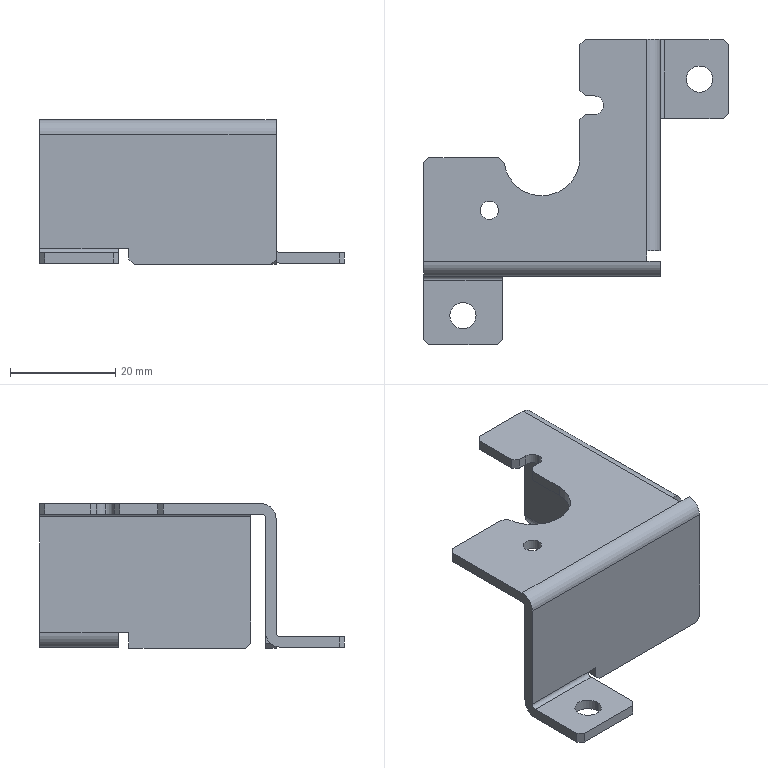Part | STEP file | AP0_JYDM_SHEET_07 | 1 solid | 60 faces | box 58 x 58 x 27.5 mm | volume 7319 mm3 | plane 43 | cylinder 17 | commonest cylinder face diameters 5 x5 3.5 x4 1.6 x3 5.6 x3 1 x1 14.5 x1